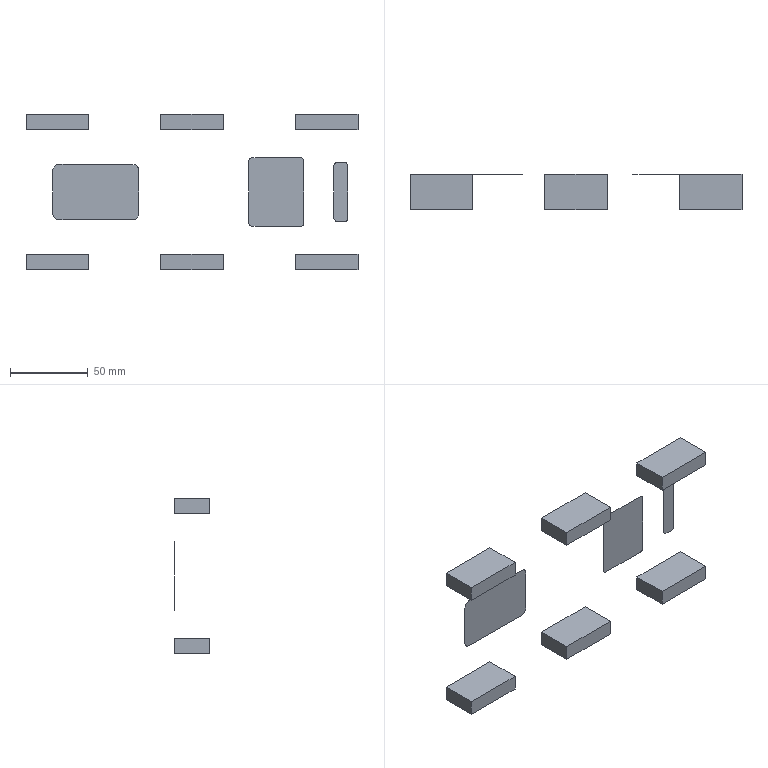Part | 6 solids | 39 faces | box 214 x 23 x 100 mm | volume 43113 mm3 | plane 36 | spline 3